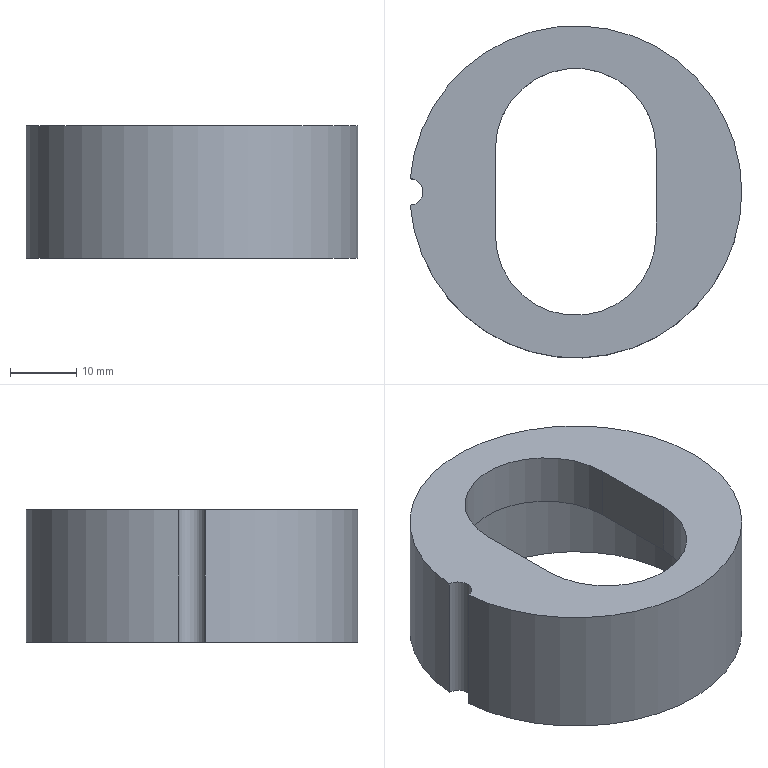Part | NX | features solid 2 | 1 solid | 10 faces | box 49.92 x 50 x 20 mm | volume 17107 mm3 | cylinder 5 | plane 5 | commonest cylinder face diameters 24.2 x2 4 x1 41 x1 50 x1
STEP:
#1=CARTESIAN_POINT('',(-249.745,-61.259,-101.));
#2=VERTEX_POINT('',#1);
#3=CARTESIAN_POINT('',(-249.745,-61.259,-81.));
#4=VERTEX_POINT('',#3);
#5=CARTESIAN_POINT('',(-249.745,-61.259,-91.));
#6=DIRECTION('',(0.,0.,1.));
#7=VECTOR('',#6,1000.);
#8=LINE('',#5,#7);
#9=EDGE_CURVE('',#2,#4,#8,.T.);
#10=ORIENTED_EDGE('',*,*,#9,.F.);
#11=CARTESIAN_POINT('',(-249.745,-57.262,-101.));
#12=VERTEX_POINT('',#11);
#13=CARTESIAN_POINT('',(-224.825,-59.26,-101.));
#14=DIRECTION('',(0.,0.,1.));
#15=DIRECTION('',(-1.,0.,0.));
#16=AXIS2_PLACEMENT_3D('',#13,#14,#15);
#17=CIRCLE('',#16,25.);
#18=EDGE_CURVE('',#2,#12,#17,.T.);
#19=ORIENTED_EDGE('',*,*,#18,.T.);
#20=CARTESIAN_POINT('',(-249.745,-57.262,-81.));
#21=VERTEX_POINT('',#20);
#22=CARTESIAN_POINT('',(-249.745,-57.262,-91.));
#23=DIRECTION('',(0.,0.,1.));
#24=VECTOR('',#23,1000.);
#25=LINE('',#22,#24);
#26=EDGE_CURVE('',#21,#12,#25,.F.);
#27=ORIENTED_EDGE('',*,*,#26,.F.);
#28=CARTESIAN_POINT('',(-224.825,-59.26,-81.));
#29=DIRECTION('',(0.,0.,1.));
#30=DIRECTION('',(-1.,0.,0.));
#31=AXIS2_PLACEMENT_3D('',#28,#29,#30);
#32=CIRCLE('',#31,25.);
#33=EDGE_CURVE('',#4,#21,#32,.T.);
#34=ORIENTED_EDGE('',*,*,#33,.F.);
#35=EDGE_LOOP('',(#10,#19,#27,#34));
#36=FACE_BOUND('',#35,.T.);
#37=CARTESIAN_POINT('',(-224.825,-59.26,-101.));
#38=DIRECTION('',(0.,0.,1.));
#39=DIRECTION('',(-1.,0.,0.));
#40=AXIS2_PLACEMENT_3D('',#37,#38,#39);
#41=CYLINDRICAL_SURFACE('',#40,25.);
#42=ADVANCED_FACE('',(#36),#41,.T.);
#43=CARTESIAN_POINT('',(-245.325,-59.26,-101.));
#44=VERTEX_POINT('',#43);
#45=CARTESIAN_POINT('',(-224.825,-59.26,-101.));
#46=DIRECTION('',(0.,0.,1.));
#47=DIRECTION('',(-1.,0.,0.));
#48=AXIS2_PLACEMENT_3D('',#45,#46,#47);
#49=CIRCLE('',#48,20.5);
#50=EDGE_CURVE('',#44,#44,#49,.T.);
#51=ORIENTED_EDGE('',*,*,#50,.T.);
#52=EDGE_LOOP('',(#51));
#53=FACE_BOUND('',#52,.T.);
#54=ORIENTED_EDGE('',*,*,#18,.F.);
#55=CARTESIAN_POINT('',(-249.825,-59.26,-101.));
#56=DIRECTION('',(0.,0.,1.));
#57=DIRECTION('',(-1.,0.,0.));
#58=AXIS2_PLACEMENT_3D('',#55,#56,#57);
#59=CIRCLE('',#58,2.);
#60=EDGE_CURVE('',#2,#12,#59,.T.);
#61=ORIENTED_EDGE('',*,*,#60,.T.);
#62=EDGE_LOOP('',(#54,#61));
#63=FACE_BOUND('',#62,.T.);
#64=CARTESIAN_POINT('',(-224.825,-59.26,-101.));
#65=DIRECTION('',(0.,0.,1.));
#66=DIRECTION('',(-1.,0.,0.));
#67=AXIS2_PLACEMENT_3D('',#64,#65,#66);
#68=PLANE('',#67);
#69=ADVANCED_FACE('',(#53,#63),#68,.F.);
#70=CARTESIAN_POINT('',(-212.725,-65.76,-81.));
#71=VERTEX_POINT('',#70);
#72=CARTESIAN_POINT('',(-212.725,-52.76,-81.));
#73=VERTEX_POINT('',#72);
#74=CARTESIAN_POINT('',(-212.725,-65.76,-81.));
#75=DIRECTION('',(0.,1.,0.));
#76=VECTOR('',#75,1000.);
#77=LINE('',#74,#76);
#78=EDGE_CURVE('',#71,#73,#77,.T.);
#79=ORIENTED_EDGE('',*,*,#78,.F.);
#80=CARTESIAN_POINT('',(-236.925,-65.76,-81.));
#81=VERTEX_POINT('',#80);
#82=CARTESIAN_POINT('',(-224.825,-65.76,-81.));
#83=DIRECTION('',(0.,0.,1.));
#84=DIRECTION('',(-1.,0.,0.));
#85=AXIS2_PLACEMENT_3D('',#82,#83,#84);
#86=CIRCLE('',#85,12.1);
#87=EDGE_CURVE('',#81,#71,#86,.T.);
#88=ORIENTED_EDGE('',*,*,#87,.F.);
#89=CARTESIAN_POINT('',(-236.925,-52.76,-81.));
#90=VERTEX_POINT('',#89);
#91=CARTESIAN_POINT('',(-236.925,-65.76,-81.));
#92=DIRECTION('',(0.,1.,0.));
#93=VECTOR('',#92,1000.);
#94=LINE('',#91,#93);
#95=EDGE_CURVE('',#81,#90,#94,.T.);
#96=ORIENTED_EDGE('',*,*,#95,.T.);
#97=CARTESIAN_POINT('',(-224.825,-52.76,-81.));
#98=DIRECTION('',(0.,0.,1.));
#99=DIRECTION('',(-1.,0.,0.));
#100=AXIS2_PLACEMENT_3D('',#97,#98,#99);
#101=CIRCLE('',#100,12.1);
#102=EDGE_CURVE('',#73,#90,#101,.T.);
#103=ORIENTED_EDGE('',*,*,#102,.F.);
#104=EDGE_LOOP('',(#79,#88,#96,#103));
#105=FACE_BOUND('',#104,.T.);
#106=CARTESIAN_POINT('',(-249.825,-59.26,-81.));
#107=DIRECTION('',(0.,0.,1.));
#108=DIRECTION('',(-1.,0.,0.));
#109=AXIS2_PLACEMENT_3D('',#106,#107,#108);
#110=CIRCLE('',#109,2.);
#111=EDGE_CURVE('',#4,#21,#110,.T.);
#112=ORIENTED_EDGE('',*,*,#111,.F.);
#113=ORIENTED_EDGE('',*,*,#33,.T.);
#114=EDGE_LOOP('',(#112,#113));
#115=FACE_BOUND('',#114,.T.);
#116=CARTESIAN_POINT('',(-224.825,-59.26,-81.));
#117=DIRECTION('',(0.,0.,1.));
#118=DIRECTION('',(-1.,0.,0.));
#119=AXIS2_PLACEMENT_3D('',#116,#117,#118);
#120=PLANE('',#119);
#121=ADVANCED_FACE('',(#105,#115),#120,.T.);
#122=ORIENTED_EDGE('',*,*,#50,.F.);
#123=EDGE_LOOP('',(#122));
#124=FACE_BOUND('',#123,.T.);
#125=CARTESIAN_POINT('',(-245.325,-59.26,-89.));
#126=VERTEX_POINT('',#125);
#127=CARTESIAN_POINT('',(-224.825,-59.26,-89.));
#128=DIRECTION('',(0.,0.,1.));
#129=DIRECTION('',(-1.,0.,0.));
#130=AXIS2_PLACEMENT_3D('',#127,#128,#129);
#131=CIRCLE('',#130,20.5);
#132=EDGE_CURVE('',#126,#126,#131,.T.);
#133=ORIENTED_EDGE('',*,*,#132,.T.);
#134=EDGE_LOOP('',(#133));
#135=FACE_BOUND('',#134,.T.);
#136=CARTESIAN_POINT('',(-224.825,-59.26,-101.));
#137=DIRECTION('',(0.,0.,1.));
#138=DIRECTION('',(-1.,0.,0.));
#139=AXIS2_PLACEMENT_3D('',#136,#137,#138);
#140=CYLINDRICAL_SURFACE('',#139,20.5);
#141=ADVANCED_FACE('',(#124,#135),#140,.F.);
#142=CARTESIAN_POINT('',(-236.925,-65.76,-89.));
#143=VERTEX_POINT('',#142);
#144=CARTESIAN_POINT('',(-212.725,-65.76,-89.));
#145=VERTEX_POINT('',#144);
#146=CARTESIAN_POINT('',(-224.825,-65.76,-89.));
#147=DIRECTION('',(0.,0.,1.));
#148=DIRECTION('',(-1.,0.,0.));
#149=AXIS2_PLACEMENT_3D('',#146,#147,#148);
#150=CIRCLE('',#149,12.1);
#151=EDGE_CURVE('',#143,#145,#150,.T.);
#152=ORIENTED_EDGE('',*,*,#151,.T.);
#153=CARTESIAN_POINT('',(-212.725,-52.76,-89.));
#154=VERTEX_POINT('',#153);
#155=CARTESIAN_POINT('',(-212.725,-59.26,-89.));
#156=DIRECTION('',(0.,1.,0.));
#157=VECTOR('',#156,1000.);
#158=LINE('',#155,#157);
#159=EDGE_CURVE('',#145,#154,#158,.T.);
#160=ORIENTED_EDGE('',*,*,#159,.T.);
#161=CARTESIAN_POINT('',(-236.925,-52.76,-89.));
#162=VERTEX_POINT('',#161);
#163=CARTESIAN_POINT('',(-224.825,-52.76,-89.));
#164=DIRECTION('',(0.,0.,1.));
#165=DIRECTION('',(-1.,0.,0.));
#166=AXIS2_PLACEMENT_3D('',#163,#164,#165);
#167=CIRCLE('',#166,12.1);
#168=EDGE_CURVE('',#154,#162,#167,.T.);
#169=ORIENTED_EDGE('',*,*,#168,.T.);
#170=CARTESIAN_POINT('',(-236.925,-59.26,-89.));
#171=DIRECTION('',(0.,1.,0.));
#172=VECTOR('',#171,1000.);
#173=LINE('',#170,#172);
#174=EDGE_CURVE('',#143,#162,#173,.T.);
#175=ORIENTED_EDGE('',*,*,#174,.F.);
#176=EDGE_LOOP('',(#152,#160,#169,#175));
#177=FACE_BOUND('',#176,.T.);
#178=ORIENTED_EDGE('',*,*,#132,.F.);
#179=EDGE_LOOP('',(#178));
#180=FACE_BOUND('',#179,.T.);
#181=CARTESIAN_POINT('',(-224.825,-59.26,-89.));
#182=DIRECTION('',(0.,0.,1.));
#183=DIRECTION('',(-1.,0.,0.));
#184=AXIS2_PLACEMENT_3D('',#181,#182,#183);
#185=PLANE('',#184);
#186=ADVANCED_FACE('',(#177,#180),#185,.F.);
#187=ORIENTED_EDGE('',*,*,#9,.T.);
#188=ORIENTED_EDGE('',*,*,#111,.T.);
#189=ORIENTED_EDGE('',*,*,#26,.T.);
#190=ORIENTED_EDGE('',*,*,#60,.F.);
#191=EDGE_LOOP('',(#187,#188,#189,#190));
#192=FACE_BOUND('',#191,.T.);
#193=CARTESIAN_POINT('',(-249.825,-59.26,-101.));
#194=DIRECTION('',(0.,0.,1.));
#195=DIRECTION('',(-1.,0.,0.));
#196=AXIS2_PLACEMENT_3D('',#193,#194,#195);
#197=CYLINDRICAL_SURFACE('',#196,2.);
#198=ADVANCED_FACE('',(#192),#197,.F.);
#199=CARTESIAN_POINT('',(-212.725,-65.76,-101.));
#200=DIRECTION('',(0.,0.,1.));
#201=VECTOR('',#200,1000.);
#202=LINE('',#199,#201);
#203=EDGE_CURVE('',#145,#71,#202,.T.);
#204=ORIENTED_EDGE('',*,*,#203,.T.);
#205=ORIENTED_EDGE('',*,*,#78,.T.);
#206=CARTESIAN_POINT('',(-212.725,-52.76,-101.));
#207=DIRECTION('',(0.,0.,1.));
#208=VECTOR('',#207,1000.);
#209=LINE('',#206,#208);
#210=EDGE_CURVE('',#154,#73,#209,.T.);
#211=ORIENTED_EDGE('',*,*,#210,.F.);
#212=ORIENTED_EDGE('',*,*,#159,.F.);
#213=EDGE_LOOP('',(#204,#205,#211,#212));
#214=FACE_BOUND('',#213,.T.);
#215=CARTESIAN_POINT('',(-212.725,-65.76,-101.));
#216=DIRECTION('',(1.,0.,0.));
#217=DIRECTION('',(0.,0.,1.));
#218=AXIS2_PLACEMENT_3D('',#215,#216,#217);
#219=PLANE('',#218);
#220=ADVANCED_FACE('',(#214),#219,.F.);
#221=ORIENTED_EDGE('',*,*,#210,.T.);
#222=ORIENTED_EDGE('',*,*,#102,.T.);
#223=CARTESIAN_POINT('',(-236.925,-52.76,-101.));
#224=DIRECTION('',(0.,0.,1.));
#225=VECTOR('',#224,1000.);
#226=LINE('',#223,#225);
#227=EDGE_CURVE('',#162,#90,#226,.T.);
#228=ORIENTED_EDGE('',*,*,#227,.F.);
#229=ORIENTED_EDGE('',*,*,#168,.F.);
#230=EDGE_LOOP('',(#221,#222,#228,#229));
#231=FACE_BOUND('',#230,.T.);
#232=CARTESIAN_POINT('',(-224.825,-52.76,-101.));
#233=DIRECTION('',(0.,0.,1.));
#234=DIRECTION('',(-1.,0.,0.));
#235=AXIS2_PLACEMENT_3D('',#232,#233,#234);
#236=CYLINDRICAL_SURFACE('',#235,12.1);
#237=ADVANCED_FACE('',(#231),#236,.F.);
#238=ORIENTED_EDGE('',*,*,#174,.T.);
#239=ORIENTED_EDGE('',*,*,#227,.T.);
#240=ORIENTED_EDGE('',*,*,#95,.F.);
#241=CARTESIAN_POINT('',(-236.925,-65.76,-101.));
#242=DIRECTION('',(0.,0.,1.));
#243=VECTOR('',#242,1000.);
#244=LINE('',#241,#243);
#245=EDGE_CURVE('',#143,#81,#244,.T.);
#246=ORIENTED_EDGE('',*,*,#245,.F.);
#247=EDGE_LOOP('',(#238,#239,#240,#246));
#248=FACE_BOUND('',#247,.T.);
#249=CARTESIAN_POINT('',(-236.925,-65.76,-101.));
#250=DIRECTION('',(1.,0.,0.));
#251=DIRECTION('',(0.,0.,1.));
#252=AXIS2_PLACEMENT_3D('',#249,#250,#251);
#253=PLANE('',#252);
#254=ADVANCED_FACE('',(#248),#253,.T.);
#255=ORIENTED_EDGE('',*,*,#245,.T.);
#256=ORIENTED_EDGE('',*,*,#87,.T.);
#257=ORIENTED_EDGE('',*,*,#203,.F.);
#258=ORIENTED_EDGE('',*,*,#151,.F.);
#259=EDGE_LOOP('',(#255,#256,#257,#258));
#260=FACE_BOUND('',#259,.T.);
#261=CARTESIAN_POINT('',(-224.825,-65.76,-101.));
#262=DIRECTION('',(0.,0.,1.));
#263=DIRECTION('',(-1.,0.,0.));
#264=AXIS2_PLACEMENT_3D('',#261,#262,#263);
#265=CYLINDRICAL_SURFACE('',#264,12.1);
#266=ADVANCED_FACE('',(#260),#265,.F.);
#267=CLOSED_SHELL('',(#42,#69,#121,#141,#186,#198,#220,#237,#254,#266));
#268=MANIFOLD_SOLID_BREP('',#267);
#269=(LENGTH_UNIT()NAMED_UNIT(*)SI_UNIT(.MILLI.,.METRE.));
#270=UNCERTAINTY_MEASURE_WITH_UNIT(LENGTH_MEASURE(0.00001),#269,'','');
#271=(NAMED_UNIT(*)PLANE_ANGLE_UNIT()SI_UNIT($,.RADIAN.));
#272=(NAMED_UNIT(*)SI_UNIT($,.STERADIAN.)SOLID_ANGLE_UNIT());
#273=(GEOMETRIC_REPRESENTATION_CONTEXT(3)GLOBAL_UNCERTAINTY_ASSIGNED_CONTEXT((#270))GLOBAL_UNIT_ASSIGNED_CONTEXT((#269,#271,#272))REPRESENTATION_CONTEXT('',''));
#274=ADVANCED_BREP_SHAPE_REPRESENTATION('',(#268),#273);